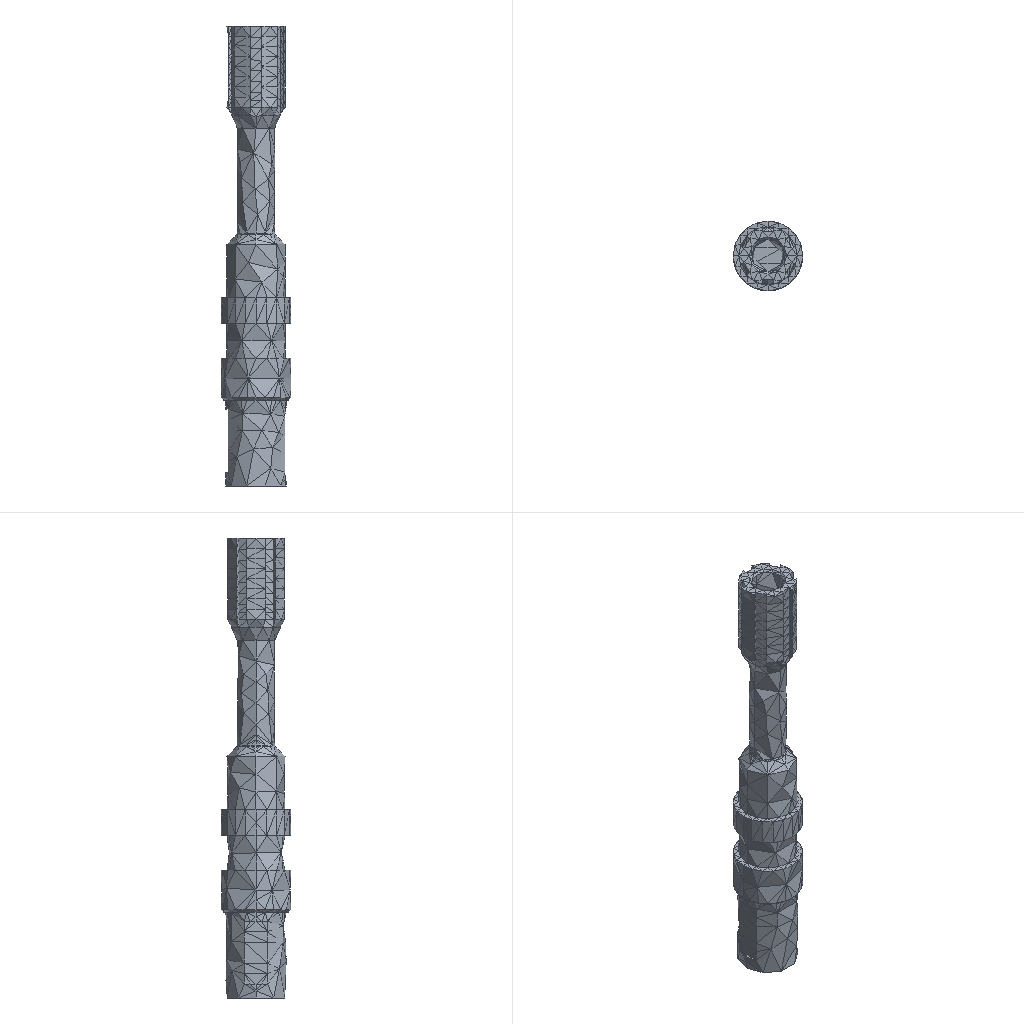Simulation study | ansys workbench
Ansys APDL input file, long lists of numbers shortened:
/batch
/config,noeldb,1     ! force off writing results to database
*get,_wallstrt,active,,time,wall
! ANSYS input file written by Workbench version 2022 R1
! File used for geometry attach: F:\ansys（分析文件汇总)\轴向柱塞泵有限元分析\轴向变量柱塞泵\轴向变量柱塞泵\驱动轴.STEP
/title,wbnew--____ (B5)
! ****** Begin Custom Load Command Snippet ******
/COM, ACT Extensions:
/COM,     LSDYNA, 2021.1
/COM,
! ****** End   Custom Load Command Snippet ******
*DIM,_wb_ProjectScratch_dir,string,248
_wb_ProjectScratch_dir(1) = 'C:\Users\Administrator\AppData\Local\Temp\WB_Administrator_15948_2\_ProjectScratch\Scr5A5D\'
*DIM,_wb_SolverFiles_dir,string,248
_wb_SolverFiles_dir(1) = 'C:\Users\Administrator\AppData\Local\Temp\WB_Administrator_15948_2\wbnew_files\dp0\SYS\MECH\'
*DIM,_wb_userfiles_dir,string,248
_wb_userfiles_dir(1) = 'C:\Users\Administrator\AppData\Local\Temp\WB_Administrator_15948_2\wbnew_files\user_files\'
/com,--- Data in consistent NMM units. See Solving Units in the help system for more information.
/units,MPA
/nopr
/wb,file,start              !  signify a WB generated input file
/prep7
! Turn off shape checking because checks already performed inside WB mesher.
! See help system for more information.
SHPP,OFF,,NOWARN
/nolist
etcon,set             ! allow ANSYS to choose best KEYOP's for 180x elements, resets any applicable keyopt to MAPDL defaults
/com,*********** Nodes for the whole assembly ***********
nblock,3,,5575
(1i9,3e20.9e3)
        1    -1.999999994E+00    -6.575305830E-08    -2.099100000E+02
! (5068 more lines like these left out)
-1
/com,*********** Nodes for all Remote Points ***********
nblock,3
(1i9,3e20.9e3)
     5070     1.573934389E-04    -4.386775707E-03    -1.188804065E+02
-1
/wb,elem,start            !  set before creation of elements
/com,*********** Elements for Body 1 "___-FreeParts|prt0003.prt.2" ***********
et,1,187
eblock,19,solid,,2686
(19i9)
        1        1        1        1        0        0        0        0       10        0        1      123      847      437      364     1636     3637     1634     1633
! (5371 more lines like these left out)
-1
/wb,elem,end               !  done creating elements
/com,*********** Send User Defined Coordinate System(s) ***********
csys,0
toffst,273.15,  ! Temperature offset from absolute zero
/com,*********** Set Reference Temperature ***********
tref,22.
/wb,mat,start              !  starting to send materials
/com,*********** Send Materials ***********
Temperature = 'TEMP' ! Temperature
MP,DENS,1,7.85e-09,	! tonne mm^-3
MP,ALPX,1,1.2e-05,	! C^-1
MP,C,1,434000000,	! mm^2 s^-2 C^-1
MP,KXX,1,60.5,	! tonne mm s^-3 C^-1
MP,RSVX,1,0.00017,	! ohm mm
MP,EX,1,200000,	! tonne s^-2 mm^-1
MP,NUXY,1,0.3,
MP,MURX,1,10000,
/wb,mat,end                !  done sending materials
!************************* Model Summary ********************
!___-FreeParts|prt0003.prt.2,	结构钢,	matid,	1
!************************* End Model Summary ********************
! get the diagonal of the bounding box. Needed later for other things
*get,_xmin,node,,mnloc,x
*get,_ymin,node,,mnloc,y
*get,_zmin,node,,mnloc,z
*get,_xmax,node,,mxloc,x
*get,_ymax,node,,mxloc,y
*get,_zmax,node,,mxloc,z
_ASMDIAG=(_xmax-_xmin)*(_xmax-_xmin)+(_ymax-_ymin)*(_ymax-_ymin)+(_zmax-_zmin)*(_zmax-_zmin)
_ASMDIAG=SQRT(_ASMDIAG)
/wb,contact,start          !  starting to send contact
/wb,contact,end            !  done creating contacts
/golist
/wb,load,start             !  starting to send loads
/com,*********** Fixed Supports ***********
CMBLOCK,_FIXEDSU,NODE,      271
(8i10)
        66        67        68        69        70        71        72       172
! (33 more lines like these left out)
cmsel,s,_FIXEDSU
d,all,all
nsel,all
/com,*********** Create Remote Point "内部远程点" ***********
! -------- Remote Point Used by "力矩" --------
*set,tid,3
*set,cid,2
et,cid,174
et,tid,170
keyo,tid,2,1               ! Don't fix the pilot node
keyo,tid,4,111111
keyo,cid,12,5              ! Bonded Contact
keyo,cid,4,1               ! Deformable RBE3 style load
keyo,cid,2,2               ! MPC style contact
eblock,10,,,246
(15i9)
     4068        2        2        2        0      489      495      494      494     3774     3800      494     3773
! (245 more lines like these left out)
-1
*set,_npilot,5070
_npilot32=_npilot
type,tid
mat ,cid
real,cid
tshape,pilo
en,4314,_npilot
tshape
/com,*********** Construct Moment Using Remote Attachment ***********
/gst,on,on
fini
*get,_numnode,node,0,count
*get,_numelem,elem,0,count
*get, _MAXELEMNUM, elem, 0, NUM, MAX
*get, _MAXNODENUM, node, 0, NUM, MAX
*get, _MAXELEMTYPE, etyp, 0, NUM, MAX
*get, _MAXREALCONST, real, 0, NUM, MAX
/go
/wb,load,end               !  done creating loads
/com,--- Number of total nodes = %_numnode%
/com,--- Number of contact elements = 246
/com,--- Number of spring elements = 0
/com,--- Number of bearing elements = 0
/com,--- Number of solid elements = 2686
/com,--- Number of condensed parts = 0
/com,--- Number of total elements = %_numelem%
*get,_wallbsol,active,,time,wall
/com,****************************************************************************
/com,*************************    SOLUTION       ********************************
/com,****************************************************************************
/solu
antype,0                   ! static analysis
_thickRatio=  1     ! Ratio of thick parts in the model
eqsl,pcg,1e-8,,,,,,1
cntr,print,1               ! print out contact info and also make no initial contact an error
dmpoption,emat,no             ! Don't combine emat file for DANSYS
dmpoption,esav,no             ! Don't combine esav file for DANSYS
nldiag,cont,iter           ! print out contact info each equilibrium iteration
rescontrol,,none                 ! Do not keep any restart files
/com,****************************************************
/com,******************* SOLVE FOR LS 1 OF 1 ****************
nsel,s,node,,5070
f,all,mx,0.
f,all,my,0.
f,all,mz,500000.
nsel,all
/nopr
/gopr
nsub,1,1,1
time,1.
outres,erase
outres,all,none
outres,nsol,all,
outres,rsol,all
outres,eangl,all
outres,etmp,all
outres,veng,all
outres,strs,all,
outres,epel,all,
outres,eppl,all,
outres,cont,all,
! *********** WB SOLVE COMMAND ***********
! check interactive state
*get,ANSINTER_,active,,int
*if,ANSINTER_,ne,0,then
/eof
*endif
solve
/com *************** Write FE CONNECTORS *********
CEWRITE,file,ce,,INTE
/com,****************************************************
/com,*************** FINISHED SOLVE FOR LS 1 *************
*get,_wallasol,active,,time,wall
/nopr
*get,_numnode,node,0,count
*get,_numelem,elem,0,count
*get, _MAXELEMNUM, elem, 0, NUM, MAX
*get, _MAXNODENUM, node, 0, NUM, MAX,,,INTERNAL
*get, _MAXELEMTYPE, etyp, 0, NUM, MAX
*get, _MAXREALCONST, real, 0, NUM, MAX
/gopr
*get,_PCGITER,active,,solu,cgiter
/post1
xmlo,ENCODING,ISO-8859-1
xmlo,parm
/xml,parm,xml
fini
/gopr
*get,_walldone,active,,time,wall
_preptime=(_wallbsol-_wallstrt)*3600
_solvtime=(_wallasol-_wallbsol)*3600
_posttime=(_walldone-_wallasol)*3600
_totaltim=(_walldone-_wallstrt)*3600
*get,_dlbratio,active,0,solu,dlbr
*get,_combtime,active,0,solu,comb
*get,_ssmode,active,0,solu,ssmm
*get,_ndofs,active,0,solu,ndof
*get,_sol_end_time,active,0,set,time
*if,_sol_end_time,eq,1.,then
/fclean				!clean distributed files
*endif
/com,--- Total number of nodes = %_numnode%
/com,--- Total number of elements = %_numelem%
/com,--- Element load balance ratio = %_dlbratio%
/com,--- Time to combine distributed files = %_combtime%
/com,--- Sparse memory mode = %_ssmode%
/com,--- Number of DOF = %_ndofs%
/wb,file,end               ! done with WB generated input